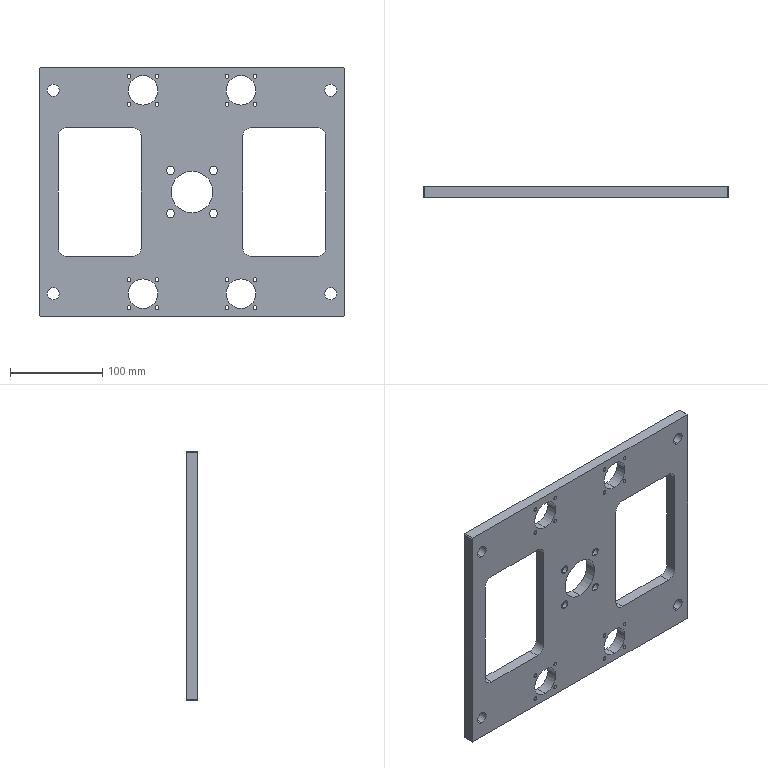Part | SolidWorks | features ICE 4, HoleWzd 3, Chamfer 1, Extrusion 1 | 1 solid | 108 faces | box 330 x 12 x 270 mm | volume 691598 mm3 | cylinder 82 | plane 26 | commonest cylinder face diameters 4.2 x32 9 x8 13 x8 15 x8 20 x8 25 x8